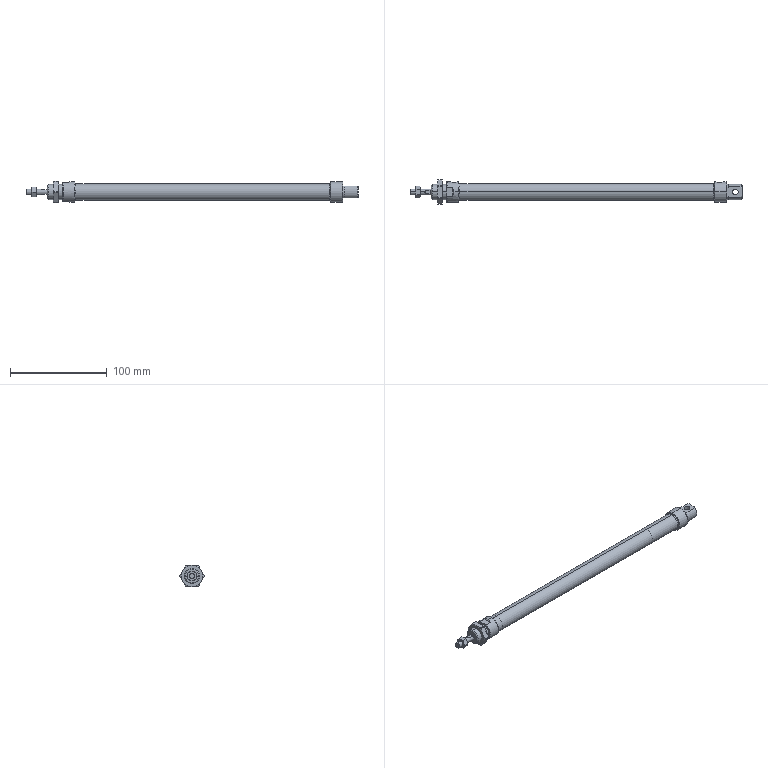Part | SolidWorks | features BaseBody 4, MoveCopyBody 2, CombineBodies 1, MoveFace 1, Split 1 | 4 solids | 138 faces | box 344 x 25 x 22 mm | volume 44525 mm3 | plane 48 | cylinder 46 | cone 36 | torus 8 | commonest cylinder face diameters 6 x6 16 x6 17.4 x6 25 x6 4.134 x4 8.5 x4